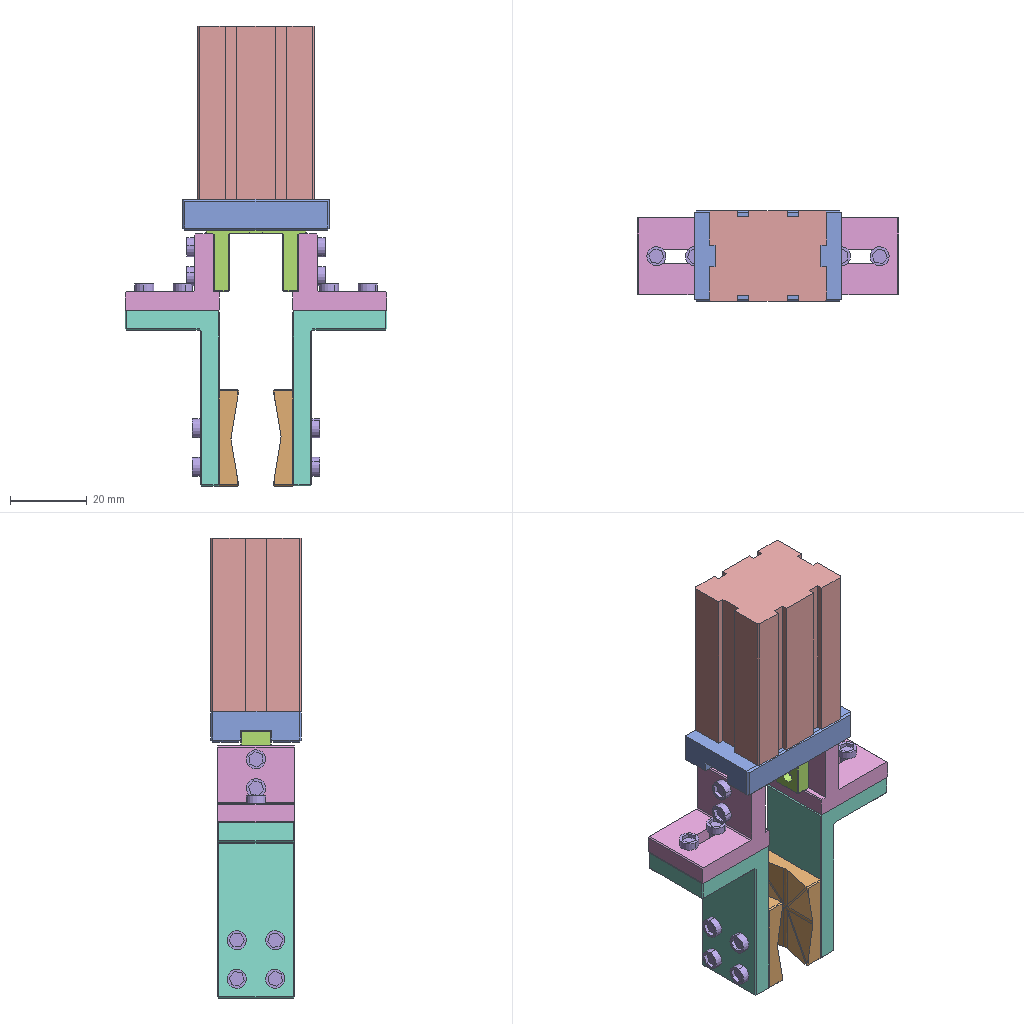Assembly | SolidWorks | 7 different items | 26 placed | box 68 x 24 x 120 mm
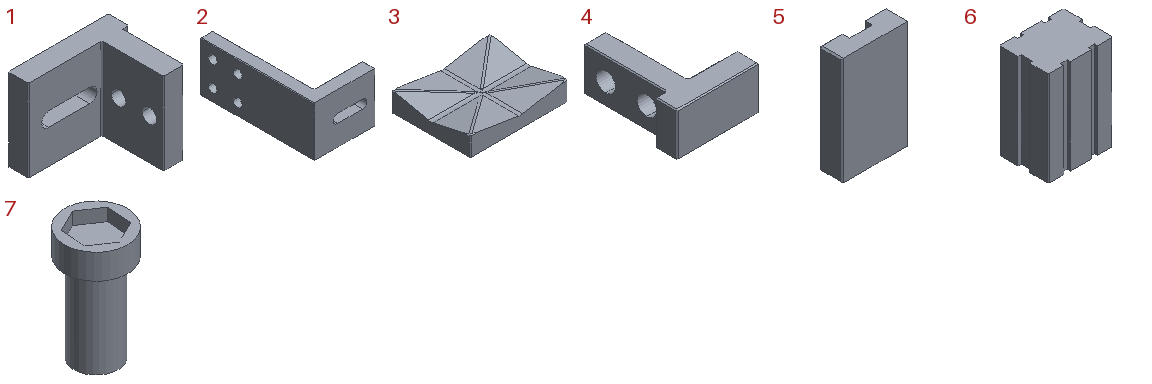Parts list (item | quantity | size | volume | features):
1 | x2 | 24.5 x 20 x 20 mm | 3626 mm3 | features ICE 2, Extrusion 1
2 | x2 | 24.5 x 45.5 x 20 mm | 6072 mm3 | features ICE 2, Chamfer 1, ExtruThin 1
3 | x2 | 25 x 20 x 4.984 mm | 1824 mm3 | features ICE 2, Chamfer 1, Extrusion 1, Fillet 1
4 | x2 | 15 x 19 x 8 mm | 879.9 mm3 | features Chamfer 1, Extrusion 1, ICE 1
5 | x1 | 23.5 x 8 x 38 mm | 6196 mm3 | features Chamfer 1, Extrusion 1
6 | x1 | 30.5 x 23.5 x 45 mm | 30669 mm3 | features Extrusion 1
7 | x16 | 5 x 5 x 9 mm | 96.197 mm3 | features ICE 2, Extrusion 1
Mates (type | each side: item.copy, entity, surface, feature):
Coincident | 6.1 face plane Boss-Extrude2 | 5.1 face plane Boss-Extrude1 | 2 times
Parallel | 6.1 face plane Boss-Extrude2 | 5.1 face plane Boss-Extrude1
Width | 5.1 face plane Boss-Extrude1 | 5.1 face plane Boss-Extrude1 | 6.1 face plane Boss-Extrude2 | 6.1 face plane Boss-Extrude2
Coincident | 5.1 face plane Boss-Extrude1 | 4.1 face plane Boss-Extrude1
Width | 5.1 face plane Boss-Extrude1 | 5.1 face plane Boss-Extrude1 | 4.1 face plane Boss-Extrude1 | 4.1 face plane Boss-Extrude1
Coincident | 5.1 face plane Boss-Extrude1 | 4.2 face plane Boss-Extrude1
Width | 5.1 face plane Boss-Extrude1 | 5.1 face plane Boss-Extrude1 | 4.2 face plane Boss-Extrude1 | 4.2 face plane Boss-Extrude1
LimitDistanceDim | 4.1 face plane Boss-Extrude1 | 5.1 face plane Boss-Extrude1
LimitDistanceDim | 4.2 face plane Boss-Extrude1 | 5.1 face plane Boss-Extrude1
Concentric | 4.1 face cylinder Cut-Extrude1 | 1.1 face cylinder Cut-Extrude2 | 2 times
Coincident | 4.1 face plane Boss-Extrude1 | 1.1 face plane Boss-Extrude1
Concentric | 4.2 face cylinder Cut-Extrude1 | 1.2 face cylinder Cut-Extrude2 | 2 times
Coincident | 4.2 face plane Boss-Extrude1 | 1.2 face plane Boss-Extrude1
Coincident | 1.1 face plane Boss-Extrude1 | 2.1 face plane Extrude-Thin1 | 3 times
Coincident | 1.2 face plane Boss-Extrude1 | 2.2 face plane Extrude-Thin1 | 3 times
Coincident | 2.2 face plane Extrude-Thin1 | 3.1 face plane Boss-Extrude1 | 3 times
Coincident | 2.1 face plane Extrude-Thin1 | 3.2 face plane Boss-Extrude1 | 3 times
Concentric | 2.2 face cylinder Cut-Extrude2 | 7.1 face cylinder Boss-Extrude2
Coincident | 2.2 face plane Extrude-Thin1 | 7.1 face plane Boss-Extrude1
Concentric | 2.2 face cylinder Cut-Extrude2 | 7.2 face cylinder Boss-Extrude2
Coincident | 2.2 face plane Extrude-Thin1 | 7.2 face plane Boss-Extrude1
Concentric | 2.2 face cylinder Cut-Extrude2 | 7.3 face cylinder Boss-Extrude2
Coincident | 2.2 face plane Extrude-Thin1 | 7.3 face plane Boss-Extrude1
Concentric | 2.2 face cylinder Cut-Extrude2 | 7.4 face cylinder Boss-Extrude2
Coincident | 2.2 face plane Extrude-Thin1 | 7.4 face plane Boss-Extrude1
Concentric | 2.1 face cylinder Cut-Extrude2 | 7.5 face cylinder Boss-Extrude2
Coincident | 2.1 face plane Extrude-Thin1 | 7.5 face plane Boss-Extrude1
Concentric | 2.1 face cylinder Cut-Extrude2 | 7.6 face cylinder Boss-Extrude2
Coincident | 2.1 face plane Extrude-Thin1 | 7.6 face plane Boss-Extrude1
Concentric | 2.1 face cylinder Cut-Extrude2 | 7.7 face cylinder Boss-Extrude2
Coincident | 2.1 face plane Extrude-Thin1 | 7.7 face plane Boss-Extrude1
Concentric | 2.1 face cylinder Cut-Extrude2 | 7.8 face cylinder Boss-Extrude2
Coincident | 2.1 face plane Extrude-Thin1 | 7.8 face plane Boss-Extrude1
Concentric | 1.2 face cylinder Cut-Extrude2 | 7.9 face cylinder Boss-Extrude2
Coincident | 1.2 face plane Boss-Extrude1 | 7.9 face plane Boss-Extrude1
Concentric | 1.2 face cylinder Cut-Extrude2 | 7.10 face cylinder Boss-Extrude2
Coincident | 1.2 face plane Boss-Extrude1 | 7.10 face plane Boss-Extrude1
Concentric | 1.1 face cylinder Cut-Extrude2 | 7.11 face cylinder Boss-Extrude2
Coincident | 1.1 face plane Boss-Extrude1 | 7.11 face plane Boss-Extrude1
Concentric | 1.1 face cylinder Cut-Extrude2 | 7.12 face cylinder Boss-Extrude2
Coincident | 1.1 face plane Boss-Extrude1 | 7.12 face plane Boss-Extrude1
Concentric | 1.1 face cylinder Cut-Extrude3 | 7.13 face cylinder Boss-Extrude2
Coincident | 1.1 face plane Boss-Extrude1 | 7.13 face plane Boss-Extrude1
Concentric | 1.1 face cylinder Cut-Extrude3 | 7.14 face cylinder Boss-Extrude2
Coincident | 1.1 face plane Boss-Extrude1 | 7.14 face plane Boss-Extrude1
Concentric | 1.2 face cylinder Cut-Extrude3 | 7.15 face cylinder Boss-Extrude2
Coincident | 1.2 face plane Boss-Extrude1 | 7.15 face plane Boss-Extrude1
Concentric | 1.2 face cylinder Cut-Extrude3 | 7.16 face cylinder Boss-Extrude2
Coincident | 1.2 face plane Boss-Extrude1 | 7.16 face plane Boss-Extrude1